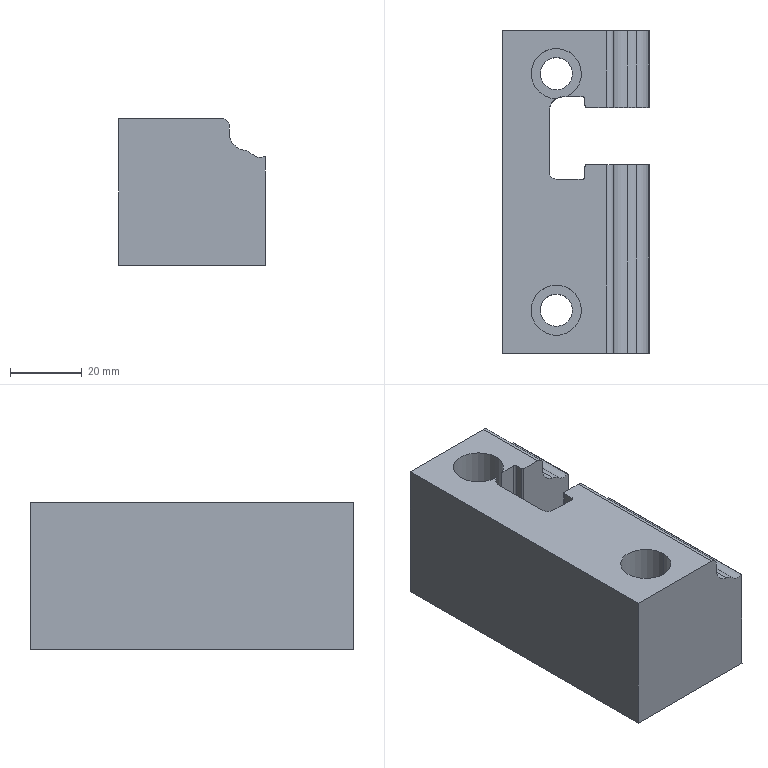Part | 1 solid | 41 faces | box 41 x 90 x 40.95 mm | volume 116029 mm3 | cylinder 23 | plane 18 | commonest cylinder face diameters 1 x4 9 x4 4 x3 14 x3 0.4 x2 6.2 x2